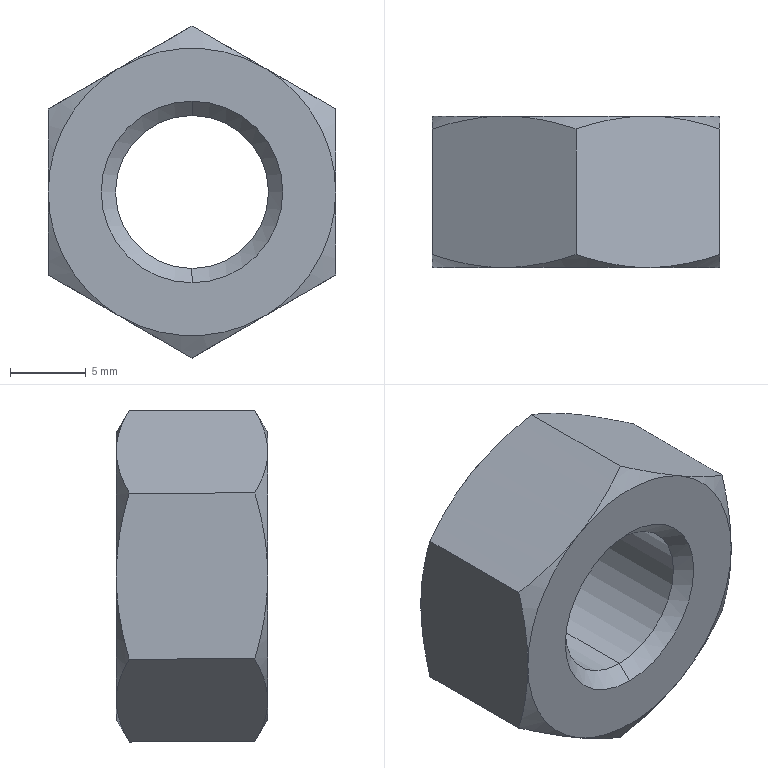Part | STEP file | JAJ_SLMNA-M12 | 1 solid | 26 faces | box 19 x 10 x 21.939 mm | volume 2279 mm3 | cone 16 | plane 8 | cylinder 2 | commonest cylinder face diameters 10.106 x2
STEP:
#1=CARTESIAN_POINT('',(-0.000000004,0.947,-5.053));
#2=VERTEX_POINT('',#1);
#3=CARTESIAN_POINT('',(0.,0.947,5.053));
#4=VERTEX_POINT('',#3);
#5=CARTESIAN_POINT('',(0.,0.947,0.));
#6=DIRECTION('',(0.,-1.,0.));
#7=DIRECTION('',(0.,0.,1.));
#8=AXIS2_PLACEMENT_3D('',#5,#6,#7);
#9=CIRCLE('',#8,5.053);
#10=EDGE_CURVE('',#2,#4,#9,.T.);
#11=ORIENTED_EDGE('',*,*,#10,.F.);
#12=CARTESIAN_POINT('',(0.,0.,-6.));
#13=VERTEX_POINT('',#12);
#14=CARTESIAN_POINT('',(0.,0.,-6.));
#15=DIRECTION('',(0.,-0.7071,-0.7071));
#16=VECTOR('',#15,1000.);
#17=LINE('',#14,#16);
#18=EDGE_CURVE('',#2,#13,#17,.T.);
#19=ORIENTED_EDGE('',*,*,#18,.T.);
#20=CARTESIAN_POINT('',(0.,0.,6.));
#21=VERTEX_POINT('',#20);
#22=CARTESIAN_POINT('',(0.,0.,0.));
#23=DIRECTION('',(0.,-1.,0.));
#24=DIRECTION('',(0.,0.,-1.));
#25=AXIS2_PLACEMENT_3D('',#22,#23,#24);
#26=CIRCLE('',#25,6.);
#27=EDGE_CURVE('',#13,#21,#26,.T.);
#28=ORIENTED_EDGE('',*,*,#27,.T.);
#29=CARTESIAN_POINT('',(0.,0.,6.));
#30=DIRECTION('',(0.,-0.7071,0.7071));
#31=VECTOR('',#30,1000.);
#32=LINE('',#29,#31);
#33=EDGE_CURVE('',#4,#21,#32,.T.);
#34=ORIENTED_EDGE('',*,*,#33,.F.);
#35=EDGE_LOOP('',(#11,#19,#28,#34));
#36=FACE_OUTER_BOUND('',#35,.T.);
#37=CARTESIAN_POINT('',(0.,0.,0.));
#38=DIRECTION('',(0.,-1.,0.));
#39=DIRECTION('',(0.,0.,1.));
#40=AXIS2_PLACEMENT_3D('',#37,#38,#39);
#41=CONICAL_SURFACE('',#40,6.,0.7854);
#42=ADVANCED_FACE('',(#36),#41,.F.);
#43=CARTESIAN_POINT('',(0.,9.053,-5.053));
#44=VERTEX_POINT('',#43);
#45=CARTESIAN_POINT('',(0.,9.053,5.053));
#46=VERTEX_POINT('',#45);
#47=CARTESIAN_POINT('',(0.,9.053,0.));
#48=DIRECTION('',(0.,-1.,0.));
#49=DIRECTION('',(0.,0.,1.));
#50=AXIS2_PLACEMENT_3D('',#47,#48,#49);
#51=CIRCLE('',#50,5.053);
#52=EDGE_CURVE('',#44,#46,#51,.T.);
#53=ORIENTED_EDGE('',*,*,#52,.F.);
#54=CARTESIAN_POINT('',(-0.000000004,0.,-5.053));
#55=DIRECTION('',(0.,-1.,0.));
#56=VECTOR('',#55,1000.);
#57=LINE('',#54,#56);
#58=EDGE_CURVE('',#44,#2,#57,.T.);
#59=ORIENTED_EDGE('',*,*,#58,.T.);
#60=ORIENTED_EDGE('',*,*,#10,.T.);
#61=CARTESIAN_POINT('',(0.000000004,0.,5.053));
#62=DIRECTION('',(0.,-1.,0.));
#63=VECTOR('',#62,1000.);
#64=LINE('',#61,#63);
#65=EDGE_CURVE('',#46,#4,#64,.T.);
#66=ORIENTED_EDGE('',*,*,#65,.F.);
#67=EDGE_LOOP('',(#53,#59,#60,#66));
#68=FACE_OUTER_BOUND('',#67,.T.);
#69=CARTESIAN_POINT('',(0.,0.,0.));
#70=DIRECTION('',(0.,-1.,0.));
#71=DIRECTION('',(0.000000001,0.,1.));
#72=AXIS2_PLACEMENT_3D('',#69,#70,#71);
#73=CYLINDRICAL_SURFACE('',#72,5.053);
#74=ADVANCED_FACE('',(#68),#73,.F.);
#75=ORIENTED_EDGE('',*,*,#52,.T.);
#76=CARTESIAN_POINT('',(0.,10.,6.));
#77=VERTEX_POINT('',#76);
#78=CARTESIAN_POINT('',(0.,10.,6.));
#79=DIRECTION('',(0.,0.7071,0.7071));
#80=VECTOR('',#79,1000.);
#81=LINE('',#78,#80);
#82=EDGE_CURVE('',#46,#77,#81,.T.);
#83=ORIENTED_EDGE('',*,*,#82,.T.);
#84=CARTESIAN_POINT('',(0.,10.,-6.));
#85=VERTEX_POINT('',#84);
#86=CARTESIAN_POINT('',(0.,10.,0.));
#87=DIRECTION('',(0.,-1.,0.));
#88=DIRECTION('',(0.,0.,1.));
#89=AXIS2_PLACEMENT_3D('',#86,#87,#88);
#90=CIRCLE('',#89,6.);
#91=EDGE_CURVE('',#85,#77,#90,.T.);
#92=ORIENTED_EDGE('',*,*,#91,.F.);
#93=CARTESIAN_POINT('',(0.,10.,-6.));
#94=DIRECTION('',(0.,0.7071,-0.7071));
#95=VECTOR('',#94,1000.);
#96=LINE('',#93,#95);
#97=EDGE_CURVE('',#44,#85,#96,.T.);
#98=ORIENTED_EDGE('',*,*,#97,.F.);
#99=EDGE_LOOP('',(#75,#83,#92,#98));
#100=FACE_OUTER_BOUND('',#99,.T.);
#101=CARTESIAN_POINT('',(0.,10.,0.));
#102=DIRECTION('',(0.,1.,0.));
#103=DIRECTION('',(0.,0.,-1.));
#104=AXIS2_PLACEMENT_3D('',#101,#102,#103);
#105=CONICAL_SURFACE('',#104,6.,0.7854);
#106=ADVANCED_FACE('',(#100),#105,.F.);
#107=CARTESIAN_POINT('',(9.5,10.,-0.0000001));
#108=VERTEX_POINT('',#107);
#109=CARTESIAN_POINT('',(9.5,9.151,-5.485));
#110=VERTEX_POINT('',#109);
#111=CARTESIAN_POINT('',(9.5,10.,-0.0000001));
#112=CARTESIAN_POINT('',(9.5,10.,-0.2425));
#113=CARTESIAN_POINT('',(9.5,9.995,-0.4848));
#114=CARTESIAN_POINT('',(9.5,9.973,-0.9718));
#115=CARTESIAN_POINT('',(9.5,9.957,-1.218));
#116=CARTESIAN_POINT('',(9.5,9.892,-1.954));
#117=CARTESIAN_POINT('',(9.5,9.832,-2.406));
#118=CARTESIAN_POINT('',(9.5,9.684,-3.298));
#119=CARTESIAN_POINT('',(9.499,9.597,-3.729));
#120=CARTESIAN_POINT('',(9.5,9.397,-4.592));
#121=CARTESIAN_POINT('',(9.5,9.284,-5.025));
#122=CARTESIAN_POINT('',(9.5,9.151,-5.485));
#123=B_SPLINE_CURVE_WITH_KNOTS('',3,(#111,#112,#113,#114,#115,#116,#117,#118,#119,#120,#121,#122),.UNSPECIFIED.,.F.,.F.,(4,2,2,2,2,4),(0.,0.125,0.25,0.5,0.75,1.),.UNSPECIFIED.);
#124=EDGE_CURVE('',#108,#110,#123,.T.);
#125=ORIENTED_EDGE('',*,*,#124,.T.);
#126=CARTESIAN_POINT('',(4.75,10.,-8.227));
#127=VERTEX_POINT('',#126);
#128=CARTESIAN_POINT('',(9.5,9.151,-5.485));
#129=CARTESIAN_POINT('',(9.094,9.287,-5.719));
#130=CARTESIAN_POINT('',(8.711,9.402,-5.939));
#131=CARTESIAN_POINT('',(7.958,9.603,-6.374));
#132=CARTESIAN_POINT('',(7.586,9.688,-6.59));
#133=CARTESIAN_POINT('',(7.011,9.798,-6.921));
#134=CARTESIAN_POINT('',(6.817,9.831,-7.033));
#135=CARTESIAN_POINT('',(6.419,9.89,-7.264));
#136=CARTESIAN_POINT('',(6.213,9.916,-7.382));
#137=CARTESIAN_POINT('',(5.582,9.979,-7.747));
#138=CARTESIAN_POINT('',(5.168,10.,-7.986));
#139=CARTESIAN_POINT('',(4.75,10.,-8.227));
#140=B_SPLINE_CURVE_WITH_KNOTS('',3,(#128,#129,#130,#131,#132,#133,#134,#135,#136,#137,#138,#139),.UNSPECIFIED.,.F.,.F.,(4,2,2,2,2,4),(0.,0.25,0.5,0.625,0.75,1.),.UNSPECIFIED.);
#141=EDGE_CURVE('',#110,#127,#140,.T.);
#142=ORIENTED_EDGE('',*,*,#141,.T.);
#143=CARTESIAN_POINT('',(0.,10.,0.));
#144=DIRECTION('',(0.,-1.,0.));
#145=DIRECTION('',(0.5,0.,-0.866));
#146=AXIS2_PLACEMENT_3D('',#143,#144,#145);
#147=CIRCLE('',#146,9.5);
#148=EDGE_CURVE('',#127,#108,#147,.T.);
#149=ORIENTED_EDGE('',*,*,#148,.T.);
#150=EDGE_LOOP('',(#125,#142,#149));
#151=FACE_OUTER_BOUND('',#150,.T.);
#152=CARTESIAN_POINT('',(0.,9.151,0.));
#153=DIRECTION('',(0.,-1.,0.));
#154=DIRECTION('',(0.5,0.,-0.866));
#155=AXIS2_PLACEMENT_3D('',#152,#153,#154);
#156=CONICAL_SURFACE('',#155,10.97,1.047);
#157=ADVANCED_FACE('',(#151),#156,.T.);
#158=CARTESIAN_POINT('',(-4.75,10.,-8.227));
#159=VERTEX_POINT('',#158);
#160=CARTESIAN_POINT('',(0.,10.,0.));
#161=DIRECTION('',(0.,-1.,0.));
#162=DIRECTION('',(-0.5,0.,-0.866));
#163=AXIS2_PLACEMENT_3D('',#160,#161,#162);
#164=CIRCLE('',#163,9.5);
#165=EDGE_CURVE('',#159,#127,#164,.T.);
#166=ORIENTED_EDGE('',*,*,#165,.T.);
#167=CARTESIAN_POINT('',(0.,9.151,-10.97));
#168=VERTEX_POINT('',#167);
#169=CARTESIAN_POINT('',(4.75,10.,-8.227));
#170=CARTESIAN_POINT('',(4.527,10.,-8.356));
#171=CARTESIAN_POINT('',(4.31,9.994,-8.482));
#172=CARTESIAN_POINT('',(3.891,9.972,-8.723));
#173=CARTESIAN_POINT('',(3.683,9.956,-8.842));
#174=CARTESIAN_POINT('',(3.262,9.913,-9.086));
#175=CARTESIAN_POINT('',(3.048,9.886,-9.209));
#176=CARTESIAN_POINT('',(2.634,9.823,-9.448));
#177=CARTESIAN_POINT('',(2.432,9.788,-9.565));
#178=CARTESIAN_POINT('',(1.839,9.672,-9.908));
#179=CARTESIAN_POINT('',(1.467,9.584,-10.122));
#180=CARTESIAN_POINT('',(0.7333,9.386,-10.545));
#181=CARTESIAN_POINT('',(0.3717,9.275,-10.755));
#182=CARTESIAN_POINT('',(0.,9.151,-10.97));
#183=B_SPLINE_CURVE_WITH_KNOTS('',3,(#169,#170,#171,#172,#173,#174,#175,#176,#177,#178,#179,#180,#181,#182),.UNSPECIFIED.,.F.,.F.,(4,2,2,2,2,2,4),(0.,0.125,0.25,0.375,0.5,0.75,1.),.UNSPECIFIED.);
#184=EDGE_CURVE('',#127,#168,#183,.T.);
#185=ORIENTED_EDGE('',*,*,#184,.T.);
#186=CARTESIAN_POINT('',(0.,9.151,-10.97));
#187=CARTESIAN_POINT('',(-0.4062,9.287,-10.735));
#188=CARTESIAN_POINT('',(-0.788,9.402,-10.514));
#189=CARTESIAN_POINT('',(-1.541,9.603,-10.079));
#190=CARTESIAN_POINT('',(-1.914,9.688,-9.865));
#191=CARTESIAN_POINT('',(-2.488,9.798,-9.533));
#192=CARTESIAN_POINT('',(-2.682,9.831,-9.421));
#193=CARTESIAN_POINT('',(-3.081,9.89,-9.191));
#194=CARTESIAN_POINT('',(-3.287,9.916,-9.072));
#195=CARTESIAN_POINT('',(-3.918,9.979,-8.708));
#196=CARTESIAN_POINT('',(-4.332,10.,-8.468));
#197=CARTESIAN_POINT('',(-4.75,10.,-8.227));
#198=B_SPLINE_CURVE_WITH_KNOTS('',3,(#186,#187,#188,#189,#190,#191,#192,#193,#194,#195,#196,#197),.UNSPECIFIED.,.F.,.F.,(4,2,2,2,2,4),(0.,0.25,0.5,0.625,0.75,1.),.UNSPECIFIED.);
#199=EDGE_CURVE('',#168,#159,#198,.T.);
#200=ORIENTED_EDGE('',*,*,#199,.T.);
#201=EDGE_LOOP('',(#166,#185,#200));
#202=FACE_OUTER_BOUND('',#201,.T.);
#203=CARTESIAN_POINT('',(0.,9.151,0.));
#204=DIRECTION('',(0.,-1.,0.));
#205=DIRECTION('',(-0.5,0.,-0.866));
#206=AXIS2_PLACEMENT_3D('',#203,#204,#205);
#207=CONICAL_SURFACE('',#206,10.97,1.047);
#208=ADVANCED_FACE('',(#202),#207,.T.);
#209=CARTESIAN_POINT('',(-9.5,10.,0.000000285));
#210=VERTEX_POINT('',#209);
#211=CARTESIAN_POINT('',(0.,10.,0.));
#212=DIRECTION('',(0.,-1.,0.));
#213=DIRECTION('',(-1.,0.,0.00000003));
#214=AXIS2_PLACEMENT_3D('',#211,#212,#213);
#215=CIRCLE('',#214,9.5);
#216=EDGE_CURVE('',#210,#159,#215,.T.);
#217=ORIENTED_EDGE('',*,*,#216,.T.);
#218=CARTESIAN_POINT('',(-9.5,9.151,-5.485));
#219=VERTEX_POINT('',#218);
#220=CARTESIAN_POINT('',(-4.75,10.,-8.227));
#221=CARTESIAN_POINT('',(-4.973,10.,-8.098));
#222=CARTESIAN_POINT('',(-5.19,9.994,-7.973));
#223=CARTESIAN_POINT('',(-5.608,9.972,-7.731));
#224=CARTESIAN_POINT('',(-5.816,9.956,-7.611));
#225=CARTESIAN_POINT('',(-6.237,9.913,-7.368));
#226=CARTESIAN_POINT('',(-6.451,9.886,-7.244));
#227=CARTESIAN_POINT('',(-6.865,9.823,-7.006));
#228=CARTESIAN_POINT('',(-7.068,9.788,-6.889));
#229=CARTESIAN_POINT('',(-7.661,9.672,-6.546));
#230=CARTESIAN_POINT('',(-8.032,9.584,-6.332));
#231=CARTESIAN_POINT('',(-8.766,9.386,-5.908));
#232=CARTESIAN_POINT('',(-9.128,9.275,-5.699));
#233=CARTESIAN_POINT('',(-9.5,9.151,-5.485));
#234=B_SPLINE_CURVE_WITH_KNOTS('',3,(#220,#221,#222,#223,#224,#225,#226,#227,#228,#229,#230,#231,#232,#233),.UNSPECIFIED.,.F.,.F.,(4,2,2,2,2,2,4),(0.,0.125,0.25,0.375,0.5,0.75,1.),.UNSPECIFIED.);
#235=EDGE_CURVE('',#159,#219,#234,.T.);
#236=ORIENTED_EDGE('',*,*,#235,.T.);
#237=CARTESIAN_POINT('',(-9.5,9.151,-5.485));
#238=CARTESIAN_POINT('',(-9.5,9.282,-5.031));
#239=CARTESIAN_POINT('',(-9.5,9.402,-4.575));
#240=CARTESIAN_POINT('',(-9.5,9.612,-3.66));
#241=CARTESIAN_POINT('',(-9.5,9.701,-3.21));
#242=CARTESIAN_POINT('',(-9.5,9.849,-2.292));
#243=CARTESIAN_POINT('',(-9.499,9.905,-1.841));
#244=CARTESIAN_POINT('',(-9.5,9.981,-0.9247));
#245=CARTESIAN_POINT('',(-9.5,10.,-0.4632));
#246=CARTESIAN_POINT('',(-9.5,10.,0.000000285));
#247=B_SPLINE_CURVE_WITH_KNOTS('',3,(#237,#238,#239,#240,#241,#242,#243,#244,#245,#246),.UNSPECIFIED.,.F.,.F.,(4,2,2,2,4),(0.,0.25,0.5,0.75,1.),.UNSPECIFIED.);
#248=EDGE_CURVE('',#219,#210,#247,.T.);
#249=ORIENTED_EDGE('',*,*,#248,.T.);
#250=EDGE_LOOP('',(#217,#236,#249));
#251=FACE_OUTER_BOUND('',#250,.T.);
#252=CARTESIAN_POINT('',(0.,9.151,0.));
#253=DIRECTION('',(0.,-1.,0.));
#254=DIRECTION('',(-1.,0.,0.00000003));
#255=AXIS2_PLACEMENT_3D('',#252,#253,#254);
#256=CONICAL_SURFACE('',#255,10.97,1.047);
#257=ADVANCED_FACE('',(#251),#256,.T.);
#258=CARTESIAN_POINT('',(4.75,10.,8.227));
#259=VERTEX_POINT('',#258);
#260=CARTESIAN_POINT('',(9.5,9.151,5.485));
#261=VERTEX_POINT('',#260);
#262=CARTESIAN_POINT('',(4.75,10.,8.227));
#263=CARTESIAN_POINT('',(4.973,10.,8.098));
#264=CARTESIAN_POINT('',(5.19,9.994,7.973));
#265=CARTESIAN_POINT('',(5.608,9.972,7.731));
#266=CARTESIAN_POINT('',(5.816,9.956,7.611));
#267=CARTESIAN_POINT('',(6.237,9.913,7.368));
#268=CARTESIAN_POINT('',(6.451,9.886,7.244));
#269=CARTESIAN_POINT('',(6.865,9.823,7.006));
#270=CARTESIAN_POINT('',(7.068,9.788,6.889));
#271=CARTESIAN_POINT('',(7.661,9.672,6.546));
#272=CARTESIAN_POINT('',(8.032,9.584,6.332));
#273=CARTESIAN_POINT('',(8.766,9.386,5.908));
#274=CARTESIAN_POINT('',(9.128,9.275,5.699));
#275=CARTESIAN_POINT('',(9.5,9.151,5.485));
#276=B_SPLINE_CURVE_WITH_KNOTS('',3,(#262,#263,#264,#265,#266,#267,#268,#269,#270,#271,#272,#273,#274,#275),.UNSPECIFIED.,.F.,.F.,(4,2,2,2,2,2,4),(0.,0.125,0.25,0.375,0.5,0.75,1.),.UNSPECIFIED.);
#277=EDGE_CURVE('',#259,#261,#276,.T.);
#278=ORIENTED_EDGE('',*,*,#277,.T.);
#279=CARTESIAN_POINT('',(9.5,9.151,5.485));
#280=CARTESIAN_POINT('',(9.5,9.282,5.031));
#281=CARTESIAN_POINT('',(9.5,9.402,4.575));
#282=CARTESIAN_POINT('',(9.5,9.612,3.66));
#283=CARTESIAN_POINT('',(9.5,9.701,3.21));
#284=CARTESIAN_POINT('',(9.5,9.849,2.292));
#285=CARTESIAN_POINT('',(9.499,9.905,1.841));
#286=CARTESIAN_POINT('',(9.5,9.981,0.9247));
#287=CARTESIAN_POINT('',(9.5,10.,0.4632));
#288=CARTESIAN_POINT('',(9.5,10.,-0.0000001));
#289=B_SPLINE_CURVE_WITH_KNOTS('',3,(#279,#280,#281,#282,#283,#284,#285,#286,#287,#288),.UNSPECIFIED.,.F.,.F.,(4,2,2,2,4),(0.,0.25,0.5,0.75,1.),.UNSPECIFIED.);
#290=EDGE_CURVE('',#261,#108,#289,.T.);
#291=ORIENTED_EDGE('',*,*,#290,.T.);
#292=CARTESIAN_POINT('',(0.,10.,0.));
#293=DIRECTION('',(0.,-1.,0.));
#294=DIRECTION('',(1.,0.,-0.000000011));
#295=AXIS2_PLACEMENT_3D('',#292,#293,#294);
#296=CIRCLE('',#295,9.5);
#297=EDGE_CURVE('',#108,#259,#296,.T.);
#298=ORIENTED_EDGE('',*,*,#297,.T.);
#299=EDGE_LOOP('',(#278,#291,#298));
#300=FACE_OUTER_BOUND('',#299,.T.);
#301=CARTESIAN_POINT('',(0.,9.151,0.));
#302=DIRECTION('',(0.,-1.,0.));
#303=DIRECTION('',(1.,0.,-0.000000011));
#304=AXIS2_PLACEMENT_3D('',#301,#302,#303);
#305=CONICAL_SURFACE('',#304,10.97,1.047);
#306=ADVANCED_FACE('',(#300),#305,.T.);
#307=CARTESIAN_POINT('',(-4.75,10.,8.227));
#308=VERTEX_POINT('',#307);
#309=CARTESIAN_POINT('',(0.,10.,0.));
#310=DIRECTION('',(0.,-1.,0.));
#311=DIRECTION('',(-0.5,0.,0.866));
#312=AXIS2_PLACEMENT_3D('',#309,#310,#311);
#313=CIRCLE('',#312,9.5);
#314=EDGE_CURVE('',#308,#210,#313,.T.);
#315=ORIENTED_EDGE('',*,*,#314,.T.);
#316=CARTESIAN_POINT('',(-9.5,9.151,5.485));
#317=VERTEX_POINT('',#316);
#318=CARTESIAN_POINT('',(-9.5,10.,0.000000285));
#319=CARTESIAN_POINT('',(-9.5,10.,0.2425));
#320=CARTESIAN_POINT('',(-9.5,9.995,0.4848));
#321=CARTESIAN_POINT('',(-9.5,9.973,0.9718));
#322=CARTESIAN_POINT('',(-9.5,9.957,1.218));
#323=CARTESIAN_POINT('',(-9.5,9.892,1.954));
#324=CARTESIAN_POINT('',(-9.5,9.832,2.406));
#325=CARTESIAN_POINT('',(-9.5,9.684,3.298));
#326=CARTESIAN_POINT('',(-9.499,9.597,3.729));
#327=CARTESIAN_POINT('',(-9.5,9.397,4.592));
#328=CARTESIAN_POINT('',(-9.5,9.284,5.025));
#329=CARTESIAN_POINT('',(-9.5,9.151,5.485));
#330=B_SPLINE_CURVE_WITH_KNOTS('',3,(#318,#319,#320,#321,#322,#323,#324,#325,#326,#327,#328,#329),.UNSPECIFIED.,.F.,.F.,(4,2,2,2,2,4),(0.,0.125,0.25,0.5,0.75,1.),.UNSPECIFIED.);
#331=EDGE_CURVE('',#210,#317,#330,.T.);
#332=ORIENTED_EDGE('',*,*,#331,.T.);
#333=CARTESIAN_POINT('',(-9.5,9.151,5.485));
#334=CARTESIAN_POINT('',(-9.094,9.287,5.719));
#335=CARTESIAN_POINT('',(-8.711,9.402,5.939));
#336=CARTESIAN_POINT('',(-7.958,9.603,6.374));
#337=CARTESIAN_POINT('',(-7.586,9.688,6.59));
#338=CARTESIAN_POINT('',(-7.011,9.798,6.921));
#339=CARTESIAN_POINT('',(-6.817,9.831,7.033));
#340=CARTESIAN_POINT('',(-6.419,9.89,7.264));
#341=CARTESIAN_POINT('',(-6.213,9.916,7.382));
#342=CARTESIAN_POINT('',(-5.582,9.979,7.747));
#343=CARTESIAN_POINT('',(-5.168,10.,7.986));
#344=CARTESIAN_POINT('',(-4.75,10.,8.227));
#345=B_SPLINE_CURVE_WITH_KNOTS('',3,(#333,#334,#335,#336,#337,#338,#339,#340,#341,#342,#343,#344),.UNSPECIFIED.,.F.,.F.,(4,2,2,2,2,4),(0.,0.25,0.5,0.625,0.75,1.),.UNSPECIFIED.);
#346=EDGE_CURVE('',#317,#308,#345,.T.);
#347=ORIENTED_EDGE('',*,*,#346,.T.);
#348=EDGE_LOOP('',(#315,#332,#347));
#349=FACE_OUTER_BOUND('',#348,.T.);
#350=CARTESIAN_POINT('',(0.,9.151,0.));
#351=DIRECTION('',(0.,-1.,0.));
#352=DIRECTION('',(-0.5,0.,0.866));
#353=AXIS2_PLACEMENT_3D('',#350,#351,#352);
#354=CONICAL_SURFACE('',#353,10.97,1.047);
#355=ADVANCED_FACE('',(#349),#354,.T.);
#356=ORIENTED_EDGE('',*,*,#297,.F.);
#357=ORIENTED_EDGE('',*,*,#148,.F.);
#358=ORIENTED_EDGE('',*,*,#165,.F.);
#359=ORIENTED_EDGE('',*,*,#216,.F.);
#360=ORIENTED_EDGE('',*,*,#314,.F.);
#361=CARTESIAN_POINT('',(0.,10.,0.));
#362=DIRECTION('',(0.,-1.,0.));
#363=DIRECTION('',(-0.5,0.,0.866));
#364=AXIS2_PLACEMENT_3D('',#361,#362,#363);
#365=CIRCLE('',#364,9.5);
#366=EDGE_CURVE('',#259,#308,#365,.T.);
#367=ORIENTED_EDGE('',*,*,#366,.F.);
#368=EDGE_LOOP('',(#356,#357,#358,#359,#360,#367));
#369=FACE_OUTER_BOUND('',#368,.T.);
#370=ORIENTED_EDGE('',*,*,#91,.T.);
#371=CARTESIAN_POINT('',(0.,10.,0.));
#372=DIRECTION('',(0.,-1.,0.));
#373=DIRECTION('',(0.,0.,1.));
#374=AXIS2_PLACEMENT_3D('',#371,#372,#373);
#375=CIRCLE('',#374,6.);
#376=EDGE_CURVE('',#77,#85,#375,.T.);
#377=ORIENTED_EDGE('',*,*,#376,.T.);
#378=EDGE_LOOP('',(#370,#377));
#379=FACE_BOUND('',#378,.T.);
#380=CARTESIAN_POINT('',(-9.5,10.,9.5));
#381=DIRECTION('',(0.,1.,0.));
#382=DIRECTION('',(1.,0.,0.));
#383=AXIS2_PLACEMENT_3D('',#380,#381,#382);
#384=PLANE('',#383);
#385=ADVANCED_FACE('',(#369,#379),#384,.T.);
#386=CARTESIAN_POINT('',(0.,9.151,10.97));
#387=VERTEX_POINT('',#386);
#388=CARTESIAN_POINT('',(-4.75,10.,8.227));
#389=CARTESIAN_POINT('',(-4.527,10.,8.356));
#390=CARTESIAN_POINT('',(-4.31,9.994,8.482));
#391=CARTESIAN_POINT('',(-3.891,9.972,8.723));
#392=CARTESIAN_POINT('',(-3.683,9.956,8.842));
#393=CARTESIAN_POINT('',(-3.262,9.913,9.086));
#394=CARTESIAN_POINT('',(-3.048,9.886,9.209));
#395=CARTESIAN_POINT('',(-2.634,9.823,9.448));
#396=CARTESIAN_POINT('',(-2.432,9.788,9.565));
#397=CARTESIAN_POINT('',(-1.839,9.672,9.908));
#398=CARTESIAN_POINT('',(-1.467,9.584,10.122));
#399=CARTESIAN_POINT('',(-0.7333,9.386,10.545));
#400=CARTESIAN_POINT('',(-0.3717,9.275,10.755));
#401=CARTESIAN_POINT('',(0.,9.151,10.97));
#402=B_SPLINE_CURVE_WITH_KNOTS('',3,(#388,#389,#390,#391,#392,#393,#394,#395,#396,#397,#398,#399,#400,#401),.UNSPECIFIED.,.F.,.F.,(4,2,2,2,2,2,4),(0.,0.125,0.25,0.375,0.5,0.75,1.),.UNSPECIFIED.);
#403=EDGE_CURVE('',#308,#387,#402,.T.);
#404=ORIENTED_EDGE('',*,*,#403,.T.);
#405=CARTESIAN_POINT('',(0.,9.151,10.97));
#406=CARTESIAN_POINT('',(0.4062,9.287,10.735));
#407=CARTESIAN_POINT('',(0.788,9.402,10.514));
#408=CARTESIAN_POINT('',(1.541,9.603,10.079));
#409=CARTESIAN_POINT('',(1.914,9.688,9.865));
#410=CARTESIAN_POINT('',(2.488,9.798,9.533));
#411=CARTESIAN_POINT('',(2.682,9.831,9.421));
#412=CARTESIAN_POINT('',(3.081,9.89,9.191));
#413=CARTESIAN_POINT('',(3.287,9.916,9.072));
#414=CARTESIAN_POINT('',(3.918,9.979,8.708));
#415=CARTESIAN_POINT('',(4.332,10.,8.468));
#416=CARTESIAN_POINT('',(4.75,10.,8.227));
#417=B_SPLINE_CURVE_WITH_KNOTS('',3,(#405,#406,#407,#408,#409,#410,#411,#412,#413,#414,#415,#416),.UNSPECIFIED.,.F.,.F.,(4,2,2,2,2,4),(0.,0.25,0.5,0.625,0.75,1.),.UNSPECIFIED.);
#418=EDGE_CURVE('',#387,#259,#417,.T.);
#419=ORIENTED_EDGE('',*,*,#418,.T.);
#420=ORIENTED_EDGE('',*,*,#366,.T.);
#421=EDGE_LOOP('',(#404,#419,#420));
#422=FACE_OUTER_BOUND('',#421,.T.);
#423=CARTESIAN_POINT('',(0.,9.151,0.));
#424=DIRECTION('',(0.,-1.,0.));
#425=DIRECTION('',(0.5,0.,0.866));
#426=AXIS2_PLACEMENT_3D('',#423,#424,#425);
#427=CONICAL_SURFACE('',#426,10.97,1.047);
#428=ADVANCED_FACE('',(#422),#427,.T.);
#429=CARTESIAN_POINT('',(-9.5,0.8485,-5.485));
#430=VERTEX_POINT('',#429);
#431=CARTESIAN_POINT('',(-9.5,9.151,-5.485));
#432=DIRECTION('',(0.,-1.,0.000000005));
#433=VECTOR('',#432,1000.);
#434=LINE('',#431,#433);
#435=EDGE_CURVE('',#219,#430,#434,.T.);
#436=ORIENTED_EDGE('',*,*,#435,.T.);
#437=CARTESIAN_POINT('',(-9.5,0.,-0.000000285));
#438=VERTEX_POINT('',#437);
#439=CARTESIAN_POINT('',(-9.5,0.,-0.000000285));
#440=CARTESIAN_POINT('',(-9.5,0.000000007,-0.2425));
#441=CARTESIAN_POINT('',(-9.5,0.005314,-0.4848));
#442=CARTESIAN_POINT('',(-9.5,0.02681,-0.9718));
#443=CARTESIAN_POINT('',(-9.5,0.04319,-1.218));
#444=CARTESIAN_POINT('',(-9.5,0.1077,-1.954));
#445=CARTESIAN_POINT('',(-9.5,0.1677,-2.406));
#446=CARTESIAN_POINT('',(-9.5,0.3159,-3.298));
#447=CARTESIAN_POINT('',(-9.499,0.4025,-3.729));
#448=CARTESIAN_POINT('',(-9.5,0.6025,-4.592));
#449=CARTESIAN_POINT('',(-9.5,0.7159,-5.025));
#450=CARTESIAN_POINT('',(-9.5,0.8485,-5.485));
#451=B_SPLINE_CURVE_WITH_KNOTS('',3,(#439,#440,#441,#442,#443,#444,#445,#446,#447,#448,#449,#450),.UNSPECIFIED.,.F.,.F.,(4,2,2,2,2,4),(0.,0.125,0.25,0.5,0.75,1.),.UNSPECIFIED.);
#452=EDGE_CURVE('',#438,#430,#451,.T.);
#453=ORIENTED_EDGE('',*,*,#452,.F.);
#454=CARTESIAN_POINT('',(-9.5,0.8485,5.485));
#455=VERTEX_POINT('',#454);
#456=CARTESIAN_POINT('',(-9.5,0.8485,5.485));
#457=CARTESIAN_POINT('',(-9.5,0.7176,5.031));
#458=CARTESIAN_POINT('',(-9.5,0.598,4.575));
#459=CARTESIAN_POINT('',(-9.5,0.388,3.66));
#460=CARTESIAN_POINT('',(-9.5,0.2991,3.21));
#461=CARTESIAN_POINT('',(-9.5,0.1514,2.292));
#462=CARTESIAN_POINT('',(-9.499,0.09541,1.841));
#463=CARTESIAN_POINT('',(-9.5,0.01949,0.9247));
#464=CARTESIAN_POINT('',(-9.5,-0.000000011,0.4632));
#465=CARTESIAN_POINT('',(-9.5,0.,-0.000000285));
#466=B_SPLINE_CURVE_WITH_KNOTS('',3,(#456,#457,#458,#459,#460,#461,#462,#463,#464,#465),.UNSPECIFIED.,.F.,.F.,(4,2,2,2,4),(0.,0.25,0.5,0.75,1.),.UNSPECIFIED.);
#467=EDGE_CURVE('',#455,#438,#466,.T.);
#468=ORIENTED_EDGE('',*,*,#467,.F.);
#469=CARTESIAN_POINT('',(-9.5,0.8485,5.485));
#470=DIRECTION('',(0.,-1.,0.000000016));
#471=VECTOR('',#470,1000.);
#472=LINE('',#469,#471);
#473=EDGE_CURVE('',#317,#455,#472,.T.);
#474=ORIENTED_EDGE('',*,*,#473,.F.);
#475=ORIENTED_EDGE('',*,*,#331,.F.);
#476=ORIENTED_EDGE('',*,*,#248,.F.);
#477=EDGE_LOOP('',(#436,#453,#468,#474,#475,#476));
#478=FACE_OUTER_BOUND('',#477,.T.);
#479=CARTESIAN_POINT('',(-9.5,-0.000000048,5.485));
#480=DIRECTION('',(-1.,0.,0.));
#481=DIRECTION('',(0.,1.,0.));
#482=AXIS2_PLACEMENT_3D('',#479,#480,#481);
#483=PLANE('',#482);
#484=ADVANCED_FACE('',(#478),#483,.T.);
#485=CARTESIAN_POINT('',(0.,0.8485,-10.97));
#486=VERTEX_POINT('',#485);
#487=CARTESIAN_POINT('',(0.,9.151,-10.97));
#488=DIRECTION('',(0.,-1.,0.));
#489=VECTOR('',#488,1000.);
#490=LINE('',#487,#489);
#491=EDGE_CURVE('',#168,#486,#490,.T.);
#492=ORIENTED_EDGE('',*,*,#491,.T.);
#493=CARTESIAN_POINT('',(-4.75,0.,-8.227));
#494=VERTEX_POINT('',#493);
#495=CARTESIAN_POINT('',(-4.75,0.,-8.227));
#496=CARTESIAN_POINT('',(-4.527,-0.000000004,-8.356));
#497=CARTESIAN_POINT('',(-4.31,0.006105,-8.482));
#498=CARTESIAN_POINT('',(-3.891,0.02785,-8.723));
#499=CARTESIAN_POINT('',(-3.683,0.04383,-8.842));
#500=CARTESIAN_POINT('',(-3.262,0.08685,-9.086));
#501=CARTESIAN_POINT('',(-3.048,0.1141,-9.209));
#502=CARTESIAN_POINT('',(-2.634,0.1767,-9.448));
#503=CARTESIAN_POINT('',(-2.432,0.2121,-9.565));
#504=CARTESIAN_POINT('',(-1.839,0.3278,-9.908));
#505=CARTESIAN_POINT('',(-1.467,0.4159,-10.122));
#506=CARTESIAN_POINT('',(-0.7333,0.614,-10.545));
#507=CARTESIAN_POINT('',(-0.3717,0.7246,-10.755));
#508=CARTESIAN_POINT('',(0.,0.8485,-10.97));
#509=B_SPLINE_CURVE_WITH_KNOTS('',3,(#495,#496,#497,#498,#499,#500,#501,#502,#503,#504,#505,#506,#507,#508),.UNSPECIFIED.,.F.,.F.,(4,2,2,2,2,2,4),(0.,0.125,0.25,0.375,0.5,0.75,1.),.UNSPECIFIED.);
#510=EDGE_CURVE('',#494,#486,#509,.T.);
#511=ORIENTED_EDGE('',*,*,#510,.F.);
#512=CARTESIAN_POINT('',(-9.5,0.8485,-5.485));
#513=CARTESIAN_POINT('',(-9.094,0.7131,-5.719));
#514=CARTESIAN_POINT('',(-8.711,0.5981,-5.939));
#515=CARTESIAN_POINT('',(-7.958,0.3973,-6.374));
#516=CARTESIAN_POINT('',(-7.586,0.3116,-6.59));
#517=CARTESIAN_POINT('',(-7.011,0.202,-6.921));
#518=CARTESIAN_POINT('',(-6.817,0.1688,-7.033));
#519=CARTESIAN_POINT('',(-6.419,0.1101,-7.264));
#520=CARTESIAN_POINT('',(-6.213,0.08437,-7.382));
#521=CARTESIAN_POINT('',(-5.582,0.02103,-7.747));
#522=CARTESIAN_POINT('',(-5.168,0.000000008,-7.986));
#523=CARTESIAN_POINT('',(-4.75,0.,-8.227));
#524=B_SPLINE_CURVE_WITH_KNOTS('',3,(#512,#513,#514,#515,#516,#517,#518,#519,#520,#521,#522,#523),.UNSPECIFIED.,.F.,.F.,(4,2,2,2,2,4),(0.,0.25,0.5,0.625,0.75,1.),.UNSPECIFIED.);
#525=EDGE_CURVE('',#430,#494,#524,.T.);
#526=ORIENTED_EDGE('',*,*,#525,.F.);
#527=ORIENTED_EDGE('',*,*,#435,.F.);
#528=ORIENTED_EDGE('',*,*,#235,.F.);
#529=ORIENTED_EDGE('',*,*,#199,.F.);
#530=EDGE_LOOP('',(#492,#511,#526,#527,#528,#529));
#531=FACE_OUTER_BOUND('',#530,.T.);
#532=CARTESIAN_POINT('',(-9.5,-0.000000032,-5.485));
#533=DIRECTION('',(-0.5,0.,-0.866));
#534=DIRECTION('',(0.,1.,0.));
#535=AXIS2_PLACEMENT_3D('',#532,#533,#534);
#536=PLANE('',#535);
#537=ADVANCED_FACE('',(#531),#536,.T.);
#538=CARTESIAN_POINT('',(9.5,0.8485,-5.485));
#539=VERTEX_POINT('',#538);
#540=CARTESIAN_POINT('',(9.5,9.151,-5.485));
#541=DIRECTION('',(-0.000000006,-1.,-0.000000003));
#542=VECTOR('',#541,1000.);
#543=LINE('',#540,#542);
#544=EDGE_CURVE('',#110,#539,#543,.T.);
#545=ORIENTED_EDGE('',*,*,#544,.T.);
#546=CARTESIAN_POINT('',(4.75,0.,-8.227));
#547=VERTEX_POINT('',#546);
#548=CARTESIAN_POINT('',(4.75,0.,-8.227));
#549=CARTESIAN_POINT('',(4.973,-0.000000004,-8.098));
#550=CARTESIAN_POINT('',(5.19,0.006105,-7.973));
#551=CARTESIAN_POINT('',(5.608,0.02785,-7.731));
#552=CARTESIAN_POINT('',(5.816,0.04383,-7.611));
#553=CARTESIAN_POINT('',(6.237,0.08685,-7.368));
#554=CARTESIAN_POINT('',(6.451,0.1141,-7.244));
#555=CARTESIAN_POINT('',(6.865,0.1767,-7.006));
#556=CARTESIAN_POINT('',(7.068,0.2121,-6.889));
#557=CARTESIAN_POINT('',(7.661,0.3278,-6.546));
#558=CARTESIAN_POINT('',(8.032,0.4159,-6.332));
#559=CARTESIAN_POINT('',(8.766,0.614,-5.908));
#560=CARTESIAN_POINT('',(9.128,0.7246,-5.699));
#561=CARTESIAN_POINT('',(9.5,0.8485,-5.485));
#562=B_SPLINE_CURVE_WITH_KNOTS('',3,(#548,#549,#550,#551,#552,#553,#554,#555,#556,#557,#558,#559,#560,#561),.UNSPECIFIED.,.F.,.F.,(4,2,2,2,2,2,4),(0.,0.125,0.25,0.375,0.5,0.75,1.),.UNSPECIFIED.);
#563=EDGE_CURVE('',#547,#539,#562,.T.);
#564=ORIENTED_EDGE('',*,*,#563,.F.);
#565=CARTESIAN_POINT('',(0.,0.8485,-10.97));
#566=CARTESIAN_POINT('',(0.4062,0.7131,-10.735));
#567=CARTESIAN_POINT('',(0.788,0.5981,-10.514));
#568=CARTESIAN_POINT('',(1.541,0.3973,-10.079));
#569=CARTESIAN_POINT('',(1.914,0.3116,-9.865));
#570=CARTESIAN_POINT('',(2.488,0.202,-9.533));
#571=CARTESIAN_POINT('',(2.682,0.1688,-9.421));
#572=CARTESIAN_POINT('',(3.081,0.1101,-9.191));
#573=CARTESIAN_POINT('',(3.287,0.08437,-9.072));
#574=CARTESIAN_POINT('',(3.918,0.02103,-8.708));
#575=CARTESIAN_POINT('',(4.332,0.000000008,-8.468));
#576=CARTESIAN_POINT('',(4.75,0.,-8.227));
#577=B_SPLINE_CURVE_WITH_KNOTS('',3,(#565,#566,#567,#568,#569,#570,#571,#572,#573,#574,#575,#576),.UNSPECIFIED.,.F.,.F.,(4,2,2,2,2,4),(0.,0.25,0.5,0.625,0.75,1.),.UNSPECIFIED.);
#578=EDGE_CURVE('',#486,#547,#577,.T.);
#579=ORIENTED_EDGE('',*,*,#578,.F.);
#580=ORIENTED_EDGE('',*,*,#491,.F.);
#581=ORIENTED_EDGE('',*,*,#184,.F.);
#582=ORIENTED_EDGE('',*,*,#141,.F.);
#583=EDGE_LOOP('',(#545,#564,#579,#580,#581,#582));
#584=FACE_OUTER_BOUND('',#583,.T.);
#585=CARTESIAN_POINT('',(0.,-0.00000003,-10.97));
#586=DIRECTION('',(0.5,0.,-0.866));
#587=DIRECTION('',(0.,1.,0.));
#588=AXIS2_PLACEMENT_3D('',#585,#586,#587);
#589=PLANE('',#588);
#590=ADVANCED_FACE('',(#584),#589,.T.);
#591=CARTESIAN_POINT('',(9.5,0.8485,5.485));
#592=VERTEX_POINT('',#591);
#593=CARTESIAN_POINT('',(9.5,9.151,5.485));
#594=DIRECTION('',(0.,-1.,-0.000000005));
#595=VECTOR('',#594,1000.);
#596=LINE('',#593,#595);
#597=EDGE_CURVE('',#261,#592,#596,.T.);
#598=ORIENTED_EDGE('',*,*,#597,.T.);
#599=CARTESIAN_POINT('',(9.5,0.,0.000000285));
#600=VERTEX_POINT('',#599);
#601=CARTESIAN_POINT('',(9.5,0.,0.000000285));
#602=CARTESIAN_POINT('',(9.5,0.000000007,0.2425));
#603=CARTESIAN_POINT('',(9.5,0.005314,0.4848));
#604=CARTESIAN_POINT('',(9.5,0.02681,0.9718));
#605=CARTESIAN_POINT('',(9.5,0.04319,1.218));
#606=CARTESIAN_POINT('',(9.5,0.1077,1.954));
#607=CARTESIAN_POINT('',(9.5,0.1677,2.406));
#608=CARTESIAN_POINT('',(9.5,0.3159,3.298));
#609=CARTESIAN_POINT('',(9.499,0.4025,3.729));
#610=CARTESIAN_POINT('',(9.5,0.6025,4.592));
#611=CARTESIAN_POINT('',(9.5,0.7159,5.025));
#612=CARTESIAN_POINT('',(9.5,0.8485,5.485));
#613=B_SPLINE_CURVE_WITH_KNOTS('',3,(#601,#602,#603,#604,#605,#606,#607,#608,#609,#610,#611,#612),.UNSPECIFIED.,.F.,.F.,(4,2,2,2,2,4),(0.,0.125,0.25,0.5,0.75,1.),.UNSPECIFIED.);
#614=EDGE_CURVE('',#600,#592,#613,.T.);
#615=ORIENTED_EDGE('',*,*,#614,.F.);
#616=CARTESIAN_POINT('',(9.5,0.8485,-5.485));
#617=CARTESIAN_POINT('',(9.5,0.7176,-5.031));
#618=CARTESIAN_POINT('',(9.5,0.598,-4.575));
#619=CARTESIAN_POINT('',(9.5,0.388,-3.66));
#620=CARTESIAN_POINT('',(9.5,0.2991,-3.21));
#621=CARTESIAN_POINT('',(9.5,0.1514,-2.292));
#622=CARTESIAN_POINT('',(9.499,0.09541,-1.841));
#623=CARTESIAN_POINT('',(9.5,0.01949,-0.9247));
#624=CARTESIAN_POINT('',(9.5,-0.000000011,-0.4632));
#625=CARTESIAN_POINT('',(9.5,0.,0.000000285));
#626=B_SPLINE_CURVE_WITH_KNOTS('',3,(#616,#617,#618,#619,#620,#621,#622,#623,#624,#625),.UNSPECIFIED.,.F.,.F.,(4,2,2,2,4),(0.,0.25,0.5,0.75,1.),.UNSPECIFIED.);
#627=EDGE_CURVE('',#539,#600,#626,.T.);
#628=ORIENTED_EDGE('',*,*,#627,.F.);
#629=ORIENTED_EDGE('',*,*,#544,.F.);
#630=ORIENTED_EDGE('',*,*,#124,.F.);
#631=ORIENTED_EDGE('',*,*,#290,.F.);
#632=EDGE_LOOP('',(#598,#615,#628,#629,#630,#631));
#633=FACE_OUTER_BOUND('',#632,.T.);
#634=CARTESIAN_POINT('',(9.5,-0.00000005,-5.485));
#635=DIRECTION('',(1.,0.,0.));
#636=DIRECTION('',(0.,1.,0.));
#637=AXIS2_PLACEMENT_3D('',#634,#635,#636);
#638=PLANE('',#637);
#639=ADVANCED_FACE('',(#633),#638,.T.);
#640=CARTESIAN_POINT('',(0.,0.8485,10.97));
#641=VERTEX_POINT('',#640);
#642=CARTESIAN_POINT('',(0.,9.151,10.97));
#643=DIRECTION('',(0.,-1.,0.));
#644=VECTOR('',#643,1000.);
#645=LINE('',#642,#644);
#646=EDGE_CURVE('',#387,#641,#645,.T.);
#647=ORIENTED_EDGE('',*,*,#646,.T.);
#648=CARTESIAN_POINT('',(4.75,0.,8.227));
#649=VERTEX_POINT('',#648);
#650=CARTESIAN_POINT('',(4.75,0.,8.227));
#651=CARTESIAN_POINT('',(4.527,-0.000000004,8.356));
#652=CARTESIAN_POINT('',(4.31,0.006105,8.482));
#653=CARTESIAN_POINT('',(3.891,0.02785,8.723));
#654=CARTESIAN_POINT('',(3.683,0.04383,8.842));
#655=CARTESIAN_POINT('',(3.262,0.08685,9.086));
#656=CARTESIAN_POINT('',(3.048,0.1141,9.209));
#657=CARTESIAN_POINT('',(2.634,0.1767,9.448));
#658=CARTESIAN_POINT('',(2.432,0.2121,9.565));
#659=CARTESIAN_POINT('',(1.839,0.3278,9.908));
#660=CARTESIAN_POINT('',(1.467,0.4159,10.122));
#661=CARTESIAN_POINT('',(0.7333,0.614,10.545));
#662=CARTESIAN_POINT('',(0.3717,0.7246,10.755));
#663=CARTESIAN_POINT('',(0.,0.8485,10.97));
#664=B_SPLINE_CURVE_WITH_KNOTS('',3,(#650,#651,#652,#653,#654,#655,#656,#657,#658,#659,#660,#661,#662,#663),.UNSPECIFIED.,.F.,.F.,(4,2,2,2,2,2,4),(0.,0.125,0.25,0.375,0.5,0.75,1.),.UNSPECIFIED.);
#665=EDGE_CURVE('',#649,#641,#664,.T.);
#666=ORIENTED_EDGE('',*,*,#665,.F.);
#667=CARTESIAN_POINT('',(9.5,0.8485,5.485));
#668=CARTESIAN_POINT('',(9.094,0.7131,5.719));
#669=CARTESIAN_POINT('',(8.711,0.5981,5.939));
#670=CARTESIAN_POINT('',(7.958,0.3973,6.374));
#671=CARTESIAN_POINT('',(7.586,0.3116,6.59));
#672=CARTESIAN_POINT('',(7.011,0.202,6.921));
#673=CARTESIAN_POINT('',(6.817,0.1688,7.033));
#674=CARTESIAN_POINT('',(6.419,0.1101,7.264));
#675=CARTESIAN_POINT('',(6.213,0.08437,7.382));
#676=CARTESIAN_POINT('',(5.582,0.02103,7.747));
#677=CARTESIAN_POINT('',(5.168,0.000000008,7.986));
#678=CARTESIAN_POINT('',(4.75,0.,8.227));
#679=B_SPLINE_CURVE_WITH_KNOTS('',3,(#667,#668,#669,#670,#671,#672,#673,#674,#675,#676,#677,#678),.UNSPECIFIED.,.F.,.F.,(4,2,2,2,2,4),(0.,0.25,0.5,0.625,0.75,1.),.UNSPECIFIED.);
#680=EDGE_CURVE('',#592,#649,#679,.T.);
#681=ORIENTED_EDGE('',*,*,#680,.F.);
#682=ORIENTED_EDGE('',*,*,#597,.F.);
#683=ORIENTED_EDGE('',*,*,#277,.F.);
#684=ORIENTED_EDGE('',*,*,#418,.F.);
#685=EDGE_LOOP('',(#647,#666,#681,#682,#683,#684));
#686=FACE_OUTER_BOUND('',#685,.T.);
#687=CARTESIAN_POINT('',(9.5,-0.000000032,5.485));
#688=DIRECTION('',(0.5,0.,0.866));
#689=DIRECTION('',(0.,1.,0.));
#690=AXIS2_PLACEMENT_3D('',#687,#688,#689);
#691=PLANE('',#690);
#692=ADVANCED_FACE('',(#686),#691,.T.);
#693=ORIENTED_EDGE('',*,*,#473,.T.);
#694=CARTESIAN_POINT('',(-4.75,0.,8.227));
#695=VERTEX_POINT('',#694);
#696=CARTESIAN_POINT('',(-4.75,0.,8.227));
#697=CARTESIAN_POINT('',(-4.973,-0.000000004,8.098));
#698=CARTESIAN_POINT('',(-5.19,0.006105,7.973));
#699=CARTESIAN_POINT('',(-5.608,0.02785,7.731));
#700=CARTESIAN_POINT('',(-5.816,0.04383,7.611));
#701=CARTESIAN_POINT('',(-6.237,0.08685,7.368));
#702=CARTESIAN_POINT('',(-6.451,0.1141,7.244));
#703=CARTESIAN_POINT('',(-6.865,0.1767,7.006));
#704=CARTESIAN_POINT('',(-7.068,0.2121,6.889));
#705=CARTESIAN_POINT('',(-7.661,0.3278,6.546));
#706=CARTESIAN_POINT('',(-8.032,0.4159,6.332));
#707=CARTESIAN_POINT('',(-8.766,0.614,5.908));
#708=CARTESIAN_POINT('',(-9.128,0.7246,5.699));
#709=CARTESIAN_POINT('',(-9.5,0.8485,5.485));
#710=B_SPLINE_CURVE_WITH_KNOTS('',3,(#696,#697,#698,#699,#700,#701,#702,#703,#704,#705,#706,#707,#708,#709),.UNSPECIFIED.,.F.,.F.,(4,2,2,2,2,2,4),(0.,0.125,0.25,0.375,0.5,0.75,1.),.UNSPECIFIED.);
#711=EDGE_CURVE('',#695,#455,#710,.T.);
#712=ORIENTED_EDGE('',*,*,#711,.F.);
#713=CARTESIAN_POINT('',(0.,0.8485,10.97));
#714=CARTESIAN_POINT('',(-0.4062,0.7131,10.735));
#715=CARTESIAN_POINT('',(-0.788,0.5981,10.514));
#716=CARTESIAN_POINT('',(-1.541,0.3973,10.079));
#717=CARTESIAN_POINT('',(-1.914,0.3116,9.865));
#718=CARTESIAN_POINT('',(-2.488,0.202,9.533));
#719=CARTESIAN_POINT('',(-2.682,0.1688,9.421));
#720=CARTESIAN_POINT('',(-3.081,0.1101,9.191));
#721=CARTESIAN_POINT('',(-3.287,0.08437,9.072));
#722=CARTESIAN_POINT('',(-3.918,0.02103,8.708));
#723=CARTESIAN_POINT('',(-4.332,0.000000008,8.468));
#724=CARTESIAN_POINT('',(-4.75,0.,8.227));
#725=B_SPLINE_CURVE_WITH_KNOTS('',3,(#713,#714,#715,#716,#717,#718,#719,#720,#721,#722,#723,#724),.UNSPECIFIED.,.F.,.F.,(4,2,2,2,2,4),(0.,0.25,0.5,0.625,0.75,1.),.UNSPECIFIED.);
#726=EDGE_CURVE('',#641,#695,#725,.T.);
#727=ORIENTED_EDGE('',*,*,#726,.F.);
#728=ORIENTED_EDGE('',*,*,#646,.F.);
#729=ORIENTED_EDGE('',*,*,#403,.F.);
#730=ORIENTED_EDGE('',*,*,#346,.F.);
#731=EDGE_LOOP('',(#693,#712,#727,#728,#729,#730));
#732=FACE_OUTER_BOUND('',#731,.T.);
#733=CARTESIAN_POINT('',(0.,-0.000000028,10.97));
#734=DIRECTION('',(-0.5,0.,0.866));
#735=DIRECTION('',(0.,1.,0.));
#736=AXIS2_PLACEMENT_3D('',#733,#734,#735);
#737=PLANE('',#736);
#738=ADVANCED_FACE('',(#732),#737,.T.);
#739=CARTESIAN_POINT('',(0.,0.,0.));
#740=DIRECTION('',(0.,-1.,0.));
#741=DIRECTION('',(1.,0.,0.00000003));
#742=AXIS2_PLACEMENT_3D('',#739,#740,#741);
#743=CIRCLE('',#742,9.5);
#744=EDGE_CURVE('',#547,#600,#743,.T.);
#745=ORIENTED_EDGE('',*,*,#744,.F.);
#746=ORIENTED_EDGE('',*,*,#563,.T.);
#747=ORIENTED_EDGE('',*,*,#627,.T.);
#748=EDGE_LOOP('',(#745,#746,#747));
#749=FACE_OUTER_BOUND('',#748,.T.);
#750=CARTESIAN_POINT('',(0.,0.8485,0.));
#751=DIRECTION('',(0.,1.,0.));
#752=DIRECTION('',(1.,0.,0.00000003));
#753=AXIS2_PLACEMENT_3D('',#750,#751,#752);
#754=CONICAL_SURFACE('',#753,10.97,1.047);
#755=ADVANCED_FACE('',(#749),#754,.T.);
#756=CARTESIAN_POINT('',(0.,0.,0.));
#757=DIRECTION('',(0.,-1.,0.));
#758=DIRECTION('',(0.5,0.,-0.866));
#759=AXIS2_PLACEMENT_3D('',#756,#757,#758);
#760=CIRCLE('',#759,9.5);
#761=EDGE_CURVE('',#494,#547,#760,.T.);
#762=ORIENTED_EDGE('',*,*,#761,.F.);
#763=ORIENTED_EDGE('',*,*,#510,.T.);
#764=ORIENTED_EDGE('',*,*,#578,.T.);
#765=EDGE_LOOP('',(#762,#763,#764));
#766=FACE_OUTER_BOUND('',#765,.T.);
#767=CARTESIAN_POINT('',(0.,0.8485,0.));
#768=DIRECTION('',(0.,1.,0.));
#769=DIRECTION('',(0.5,0.,-0.866));
#770=AXIS2_PLACEMENT_3D('',#767,#768,#769);
#771=CONICAL_SURFACE('',#770,10.97,1.047);
#772=ADVANCED_FACE('',(#766),#771,.T.);
#773=CARTESIAN_POINT('',(0.,0.,0.));
#774=DIRECTION('',(0.,-1.,0.));
#775=DIRECTION('',(-0.5,0.,-0.866));
#776=AXIS2_PLACEMENT_3D('',#773,#774,#775);
#777=CIRCLE('',#776,9.5);
#778=EDGE_CURVE('',#438,#494,#777,.T.);
#779=ORIENTED_EDGE('',*,*,#778,.F.);
#780=ORIENTED_EDGE('',*,*,#452,.T.);
#781=ORIENTED_EDGE('',*,*,#525,.T.);
#782=EDGE_LOOP('',(#779,#780,#781));
#783=FACE_OUTER_BOUND('',#782,.T.);
#784=CARTESIAN_POINT('',(0.,0.8485,0.));
#785=DIRECTION('',(0.,1.,0.));
#786=DIRECTION('',(-0.5,0.,-0.866));
#787=AXIS2_PLACEMENT_3D('',#784,#785,#786);
#788=CONICAL_SURFACE('',#787,10.97,1.047);
#789=ADVANCED_FACE('',(#783),#788,.T.);
#790=CARTESIAN_POINT('',(0.,0.,0.));
#791=DIRECTION('',(0.,-1.,0.));
#792=DIRECTION('',(-0.5,0.,0.866));
#793=AXIS2_PLACEMENT_3D('',#790,#791,#792);
#794=CIRCLE('',#793,9.5);
#795=EDGE_CURVE('',#649,#695,#794,.T.);
#796=ORIENTED_EDGE('',*,*,#795,.F.);
#797=ORIENTED_EDGE('',*,*,#665,.T.);
#798=ORIENTED_EDGE('',*,*,#726,.T.);
#799=EDGE_LOOP('',(#796,#797,#798));
#800=FACE_OUTER_BOUND('',#799,.T.);
#801=CARTESIAN_POINT('',(0.,0.8485,0.));
#802=DIRECTION('',(0.,1.,0.));
#803=DIRECTION('',(-0.5,0.,0.866));
#804=AXIS2_PLACEMENT_3D('',#801,#802,#803);
#805=CONICAL_SURFACE('',#804,10.97,1.047);
#806=ADVANCED_FACE('',(#800),#805,.T.);
#807=CARTESIAN_POINT('',(0.,0.,0.));
#808=DIRECTION('',(0.,-1.,0.));
#809=DIRECTION('',(0.5,0.,0.866));
#810=AXIS2_PLACEMENT_3D('',#807,#808,#809);
#811=CIRCLE('',#810,9.5);
#812=EDGE_CURVE('',#600,#649,#811,.T.);
#813=ORIENTED_EDGE('',*,*,#812,.F.);
#814=ORIENTED_EDGE('',*,*,#614,.T.);
#815=ORIENTED_EDGE('',*,*,#680,.T.);
#816=EDGE_LOOP('',(#813,#814,#815));
#817=FACE_OUTER_BOUND('',#816,.T.);
#818=CARTESIAN_POINT('',(0.,0.8485,0.));
#819=DIRECTION('',(0.,1.,0.));
#820=DIRECTION('',(0.5,0.,0.866));
#821=AXIS2_PLACEMENT_3D('',#818,#819,#820);
#822=CONICAL_SURFACE('',#821,10.97,1.047);
#823=ADVANCED_FACE('',(#817),#822,.T.);
#824=ORIENTED_EDGE('',*,*,#744,.T.);
#825=ORIENTED_EDGE('',*,*,#812,.T.);
#826=ORIENTED_EDGE('',*,*,#795,.T.);
#827=CARTESIAN_POINT('',(0.,0.,0.));
#828=DIRECTION('',(0.,-1.,0.));
#829=DIRECTION('',(-0.5,0.,0.866));
#830=AXIS2_PLACEMENT_3D('',#827,#828,#829);
#831=CIRCLE('',#830,9.5);
#832=EDGE_CURVE('',#695,#438,#831,.T.);
#833=ORIENTED_EDGE('',*,*,#832,.T.);
#834=ORIENTED_EDGE('',*,*,#778,.T.);
#835=ORIENTED_EDGE('',*,*,#761,.T.);
#836=EDGE_LOOP('',(#824,#825,#826,#833,#834,#835));
#837=FACE_OUTER_BOUND('',#836,.T.);
#838=CARTESIAN_POINT('',(0.,0.,0.));
#839=DIRECTION('',(0.,-1.,0.));
#840=DIRECTION('',(0.,0.,-1.));
#841=AXIS2_PLACEMENT_3D('',#838,#839,#840);
#842=CIRCLE('',#841,6.);
#843=EDGE_CURVE('',#21,#13,#842,.T.);
#844=ORIENTED_EDGE('',*,*,#843,.F.);
#845=ORIENTED_EDGE('',*,*,#27,.F.);
#846=EDGE_LOOP('',(#844,#845));
#847=FACE_BOUND('',#846,.T.);
#848=CARTESIAN_POINT('',(-9.5,0.,-9.5));
#849=DIRECTION('',(0.,-1.,0.));
#850=DIRECTION('',(1.,0.,0.));
#851=AXIS2_PLACEMENT_3D('',#848,#849,#850);
#852=PLANE('',#851);
#853=ADVANCED_FACE('',(#837,#847),#852,.T.);
#854=ORIENTED_EDGE('',*,*,#711,.T.);
#855=ORIENTED_EDGE('',*,*,#467,.T.);
#856=ORIENTED_EDGE('',*,*,#832,.F.);
#857=EDGE_LOOP('',(#854,#855,#856));
#858=FACE_OUTER_BOUND('',#857,.T.);
#859=CARTESIAN_POINT('',(0.,0.8485,0.));
#860=DIRECTION('',(0.,1.,0.));
#861=DIRECTION('',(-1.,0.,-0.00000003));
#862=AXIS2_PLACEMENT_3D('',#859,#860,#861);
#863=CONICAL_SURFACE('',#862,10.97,1.047);
#864=ADVANCED_FACE('',(#858),#863,.T.);
#865=ORIENTED_EDGE('',*,*,#82,.F.);
#866=CARTESIAN_POINT('',(0.,9.053,0.));
#867=DIRECTION('',(0.,-1.,0.));
#868=DIRECTION('',(0.,0.,1.));
#869=AXIS2_PLACEMENT_3D('',#866,#867,#868);
#870=CIRCLE('',#869,5.053);
#871=EDGE_CURVE('',#46,#44,#870,.T.);
#872=ORIENTED_EDGE('',*,*,#871,.T.);
#873=ORIENTED_EDGE('',*,*,#97,.T.);
#874=ORIENTED_EDGE('',*,*,#376,.F.);
#875=EDGE_LOOP('',(#865,#872,#873,#874));
#876=FACE_OUTER_BOUND('',#875,.T.);
#877=CARTESIAN_POINT('',(0.,10.,0.));
#878=DIRECTION('',(0.,1.,0.));
#879=DIRECTION('',(0.,0.,-1.));
#880=AXIS2_PLACEMENT_3D('',#877,#878,#879);
#881=CONICAL_SURFACE('',#880,6.,0.7854);
#882=ADVANCED_FACE('',(#876),#881,.F.);
#883=ORIENTED_EDGE('',*,*,#58,.F.);
#884=ORIENTED_EDGE('',*,*,#871,.F.);
#885=ORIENTED_EDGE('',*,*,#65,.T.);
#886=CARTESIAN_POINT('',(0.,0.947,0.));
#887=DIRECTION('',(0.,-1.,0.));
#888=DIRECTION('',(0.,0.,1.));
#889=AXIS2_PLACEMENT_3D('',#886,#887,#888);
#890=CIRCLE('',#889,5.053);
#891=EDGE_CURVE('',#4,#2,#890,.T.);
#892=ORIENTED_EDGE('',*,*,#891,.T.);
#893=EDGE_LOOP('',(#883,#884,#885,#892));
#894=FACE_OUTER_BOUND('',#893,.T.);
#895=CARTESIAN_POINT('',(0.,0.,0.));
#896=DIRECTION('',(0.,-1.,0.));
#897=DIRECTION('',(0.000000001,0.,1.));
#898=AXIS2_PLACEMENT_3D('',#895,#896,#897);
#899=CYLINDRICAL_SURFACE('',#898,5.053);
#900=ADVANCED_FACE('',(#894),#899,.F.);
#901=ORIENTED_EDGE('',*,*,#18,.F.);
#902=ORIENTED_EDGE('',*,*,#891,.F.);
#903=ORIENTED_EDGE('',*,*,#33,.T.);
#904=ORIENTED_EDGE('',*,*,#843,.T.);
#905=EDGE_LOOP('',(#901,#902,#903,#904));
#906=FACE_OUTER_BOUND('',#905,.T.);
#907=CARTESIAN_POINT('',(0.,0.,0.));
#908=DIRECTION('',(0.,-1.,0.));
#909=DIRECTION('',(0.,0.,1.));
#910=AXIS2_PLACEMENT_3D('',#907,#908,#909);
#911=CONICAL_SURFACE('',#910,6.,0.7854);
#912=ADVANCED_FACE('',(#906),#911,.F.);
#913=CLOSED_SHELL('',(#42,#74,#106,#157,#208,#257,#306,#355,#385,#428,#484,#537,#590,#639,#692,#738,#755,#772,#789,#806,#823,#853,#864,#882,#900,#912));
#914=MANIFOLD_SOLID_BREP('',#913);
#915=CARTESIAN_POINT('',(0.,0.,0.));
#916=DIRECTION('',(0.,0.,1.));
#917=DIRECTION('',(1.,0.,0.));
#918=AXIS2_PLACEMENT_3D('',#915,#916,#917);
#919=(LENGTH_UNIT()NAMED_UNIT(*)SI_UNIT(.MILLI.,.METRE.));
#920=UNCERTAINTY_MEASURE_WITH_UNIT(LENGTH_MEASURE(0.00001),#919,'','');
#921=(NAMED_UNIT(*)PLANE_ANGLE_UNIT()SI_UNIT($,.RADIAN.));
#922=(NAMED_UNIT(*)SI_UNIT($,.STERADIAN.)SOLID_ANGLE_UNIT());
#923=(GEOMETRIC_REPRESENTATION_CONTEXT(3)GLOBAL_UNCERTAINTY_ASSIGNED_CONTEXT((#920))GLOBAL_UNIT_ASSIGNED_CONTEXT((#919,#921,#922))REPRESENTATION_CONTEXT('',''));
#924=ADVANCED_BREP_SHAPE_REPRESENTATION('',(#914,#918),#923);